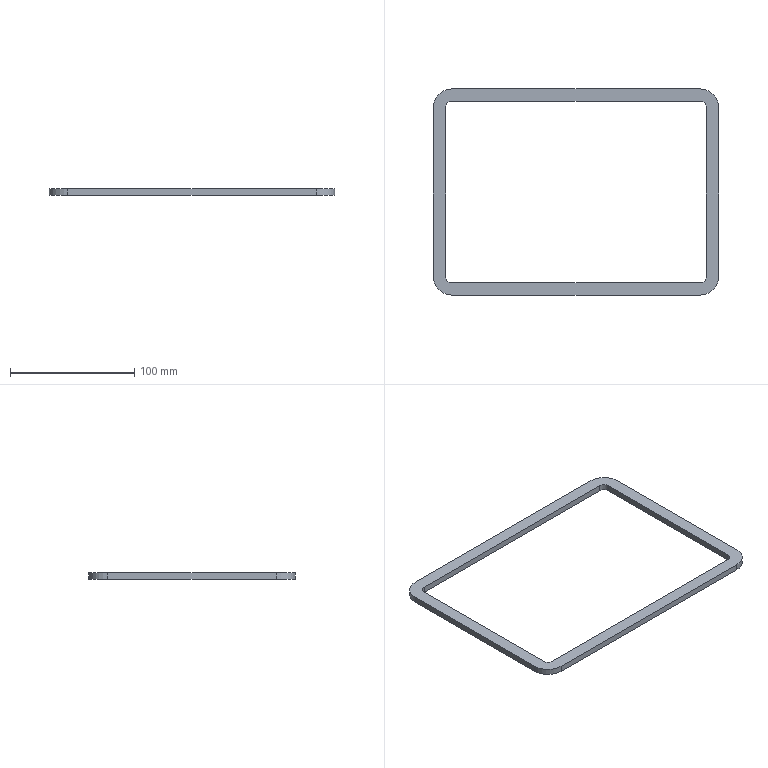Part | SolidWorks | features Fillet 2, Extrusion 1 | 1 solid | 18 faces | box 230 x 166 x 5 mm | volume 36742 mm3 | plane 10 | cylinder 8 | commonest cylinder face diameters 10 x4 30 x4
STEP:
#1=CARTESIAN_POINT('',(-100.,-83.,5.));
#2=VERTEX_POINT('',#1);
#3=CARTESIAN_POINT('',(100.,-83.,5.));
#4=VERTEX_POINT('',#3);
#5=CARTESIAN_POINT('',(-115.,-83.,5.));
#6=DIRECTION('',(1.,0.,0.));
#7=VECTOR('',#6,1000.);
#8=LINE('',#5,#7);
#9=EDGE_CURVE('',#2,#4,#8,.T.);
#10=ORIENTED_EDGE('',*,*,#9,.T.);
#11=CARTESIAN_POINT('',(115.,-68.,5.));
#12=VERTEX_POINT('',#11);
#13=CARTESIAN_POINT('',(100.,-68.,5.));
#14=DIRECTION('',(0.,0.,1.));
#15=DIRECTION('',(1.,0.,0.));
#16=AXIS2_PLACEMENT_3D('',#13,#14,#15);
#17=CIRCLE('',#16,15.);
#18=EDGE_CURVE('',#4,#12,#17,.T.);
#19=ORIENTED_EDGE('',*,*,#18,.T.);
#20=CARTESIAN_POINT('',(115.,68.,5.));
#21=VERTEX_POINT('',#20);
#22=CARTESIAN_POINT('',(115.,83.,5.));
#23=DIRECTION('',(0.,1.,0.));
#24=VECTOR('',#23,1000.);
#25=LINE('',#22,#24);
#26=EDGE_CURVE('',#12,#21,#25,.T.);
#27=ORIENTED_EDGE('',*,*,#26,.T.);
#28=CARTESIAN_POINT('',(100.,83.,5.));
#29=VERTEX_POINT('',#28);
#30=CARTESIAN_POINT('',(100.,68.,5.));
#31=DIRECTION('',(0.,0.,1.));
#32=DIRECTION('',(1.,0.,0.));
#33=AXIS2_PLACEMENT_3D('',#30,#31,#32);
#34=CIRCLE('',#33,15.);
#35=EDGE_CURVE('',#21,#29,#34,.T.);
#36=ORIENTED_EDGE('',*,*,#35,.T.);
#37=CARTESIAN_POINT('',(-100.,83.,5.));
#38=VERTEX_POINT('',#37);
#39=CARTESIAN_POINT('',(-115.,83.,5.));
#40=DIRECTION('',(-1.,0.,0.));
#41=VECTOR('',#40,1000.);
#42=LINE('',#39,#41);
#43=EDGE_CURVE('',#29,#38,#42,.T.);
#44=ORIENTED_EDGE('',*,*,#43,.T.);
#45=CARTESIAN_POINT('',(-115.,68.,5.));
#46=VERTEX_POINT('',#45);
#47=CARTESIAN_POINT('',(-100.,68.,5.));
#48=DIRECTION('',(0.,0.,1.));
#49=DIRECTION('',(1.,0.,0.));
#50=AXIS2_PLACEMENT_3D('',#47,#48,#49);
#51=CIRCLE('',#50,15.);
#52=EDGE_CURVE('',#38,#46,#51,.T.);
#53=ORIENTED_EDGE('',*,*,#52,.T.);
#54=CARTESIAN_POINT('',(-115.,-68.,5.));
#55=VERTEX_POINT('',#54);
#56=CARTESIAN_POINT('',(-115.,83.,5.));
#57=DIRECTION('',(0.,-1.,0.));
#58=VECTOR('',#57,1000.);
#59=LINE('',#56,#58);
#60=EDGE_CURVE('',#46,#55,#59,.T.);
#61=ORIENTED_EDGE('',*,*,#60,.T.);
#62=CARTESIAN_POINT('',(-100.,-68.,5.));
#63=DIRECTION('',(0.,0.,1.));
#64=DIRECTION('',(1.,0.,0.));
#65=AXIS2_PLACEMENT_3D('',#62,#63,#64);
#66=CIRCLE('',#65,15.);
#67=EDGE_CURVE('',#55,#2,#66,.T.);
#68=ORIENTED_EDGE('',*,*,#67,.T.);
#69=EDGE_LOOP('',(#10,#19,#27,#36,#44,#53,#61,#68));
#70=FACE_OUTER_BOUND('',#69,.T.);
#71=CARTESIAN_POINT('',(-100.,-73.,5.));
#72=VERTEX_POINT('',#71);
#73=CARTESIAN_POINT('',(100.,-73.,5.));
#74=VERTEX_POINT('',#73);
#75=CARTESIAN_POINT('',(-105.,-73.,5.));
#76=DIRECTION('',(1.,0.,0.));
#77=VECTOR('',#76,1000.);
#78=LINE('',#75,#77);
#79=EDGE_CURVE('',#72,#74,#78,.T.);
#80=ORIENTED_EDGE('',*,*,#79,.F.);
#81=CARTESIAN_POINT('',(-105.,-68.,5.));
#82=VERTEX_POINT('',#81);
#83=CARTESIAN_POINT('',(-100.,-68.,5.));
#84=DIRECTION('',(0.,0.,-1.));
#85=DIRECTION('',(1.,0.,0.));
#86=AXIS2_PLACEMENT_3D('',#83,#84,#85);
#87=CIRCLE('',#86,5.);
#88=EDGE_CURVE('',#72,#82,#87,.T.);
#89=ORIENTED_EDGE('',*,*,#88,.T.);
#90=CARTESIAN_POINT('',(-105.,68.,5.));
#91=VERTEX_POINT('',#90);
#92=CARTESIAN_POINT('',(-105.,73.,5.));
#93=DIRECTION('',(0.,-1.,0.));
#94=VECTOR('',#93,1000.);
#95=LINE('',#92,#94);
#96=EDGE_CURVE('',#91,#82,#95,.T.);
#97=ORIENTED_EDGE('',*,*,#96,.F.);
#98=CARTESIAN_POINT('',(-100.,73.,5.));
#99=VERTEX_POINT('',#98);
#100=CARTESIAN_POINT('',(-100.,68.,5.));
#101=DIRECTION('',(0.,0.,-1.));
#102=DIRECTION('',(1.,0.,0.));
#103=AXIS2_PLACEMENT_3D('',#100,#101,#102);
#104=CIRCLE('',#103,5.);
#105=EDGE_CURVE('',#91,#99,#104,.T.);
#106=ORIENTED_EDGE('',*,*,#105,.T.);
#107=CARTESIAN_POINT('',(100.,73.,5.));
#108=VERTEX_POINT('',#107);
#109=CARTESIAN_POINT('',(-105.,73.,5.));
#110=DIRECTION('',(-1.,0.,0.));
#111=VECTOR('',#110,1000.);
#112=LINE('',#109,#111);
#113=EDGE_CURVE('',#108,#99,#112,.T.);
#114=ORIENTED_EDGE('',*,*,#113,.F.);
#115=CARTESIAN_POINT('',(105.,68.,5.));
#116=VERTEX_POINT('',#115);
#117=CARTESIAN_POINT('',(100.,68.,5.));
#118=DIRECTION('',(0.,0.,-1.));
#119=DIRECTION('',(1.,0.,0.));
#120=AXIS2_PLACEMENT_3D('',#117,#118,#119);
#121=CIRCLE('',#120,5.);
#122=EDGE_CURVE('',#108,#116,#121,.T.);
#123=ORIENTED_EDGE('',*,*,#122,.T.);
#124=CARTESIAN_POINT('',(105.,-68.,5.));
#125=VERTEX_POINT('',#124);
#126=CARTESIAN_POINT('',(105.,73.,5.));
#127=DIRECTION('',(0.,1.,0.));
#128=VECTOR('',#127,1000.);
#129=LINE('',#126,#128);
#130=EDGE_CURVE('',#125,#116,#129,.T.);
#131=ORIENTED_EDGE('',*,*,#130,.F.);
#132=CARTESIAN_POINT('',(100.,-68.,5.));
#133=DIRECTION('',(0.,0.,-1.));
#134=DIRECTION('',(1.,0.,0.));
#135=AXIS2_PLACEMENT_3D('',#132,#133,#134);
#136=CIRCLE('',#135,5.);
#137=EDGE_CURVE('',#125,#74,#136,.T.);
#138=ORIENTED_EDGE('',*,*,#137,.T.);
#139=EDGE_LOOP('',(#80,#89,#97,#106,#114,#123,#131,#138));
#140=FACE_BOUND('',#139,.T.);
#141=CARTESIAN_POINT('',(0.,0.,5.));
#142=DIRECTION('',(0.,0.,1.));
#143=DIRECTION('',(1.,0.,0.));
#144=AXIS2_PLACEMENT_3D('',#141,#142,#143);
#145=PLANE('',#144);
#146=ADVANCED_FACE('',(#70,#140),#145,.T.);
#147=CARTESIAN_POINT('',(115.,-68.,0.));
#148=VERTEX_POINT('',#147);
#149=CARTESIAN_POINT('',(115.,68.,0.));
#150=VERTEX_POINT('',#149);
#151=CARTESIAN_POINT('',(115.,83.,0.));
#152=DIRECTION('',(0.,1.,0.));
#153=VECTOR('',#152,1000.);
#154=LINE('',#151,#153);
#155=EDGE_CURVE('',#148,#150,#154,.T.);
#156=ORIENTED_EDGE('',*,*,#155,.F.);
#157=CARTESIAN_POINT('',(100.,-83.,0.));
#158=VERTEX_POINT('',#157);
#159=CARTESIAN_POINT('',(100.,-68.,0.));
#160=DIRECTION('',(0.,0.,-1.));
#161=DIRECTION('',(1.,0.,0.));
#162=AXIS2_PLACEMENT_3D('',#159,#160,#161);
#163=CIRCLE('',#162,15.);
#164=EDGE_CURVE('',#148,#158,#163,.T.);
#165=ORIENTED_EDGE('',*,*,#164,.T.);
#166=CARTESIAN_POINT('',(-100.,-83.,0.));
#167=VERTEX_POINT('',#166);
#168=CARTESIAN_POINT('',(-115.,-83.,0.));
#169=DIRECTION('',(1.,0.,0.));
#170=VECTOR('',#169,1000.);
#171=LINE('',#168,#170);
#172=EDGE_CURVE('',#167,#158,#171,.T.);
#173=ORIENTED_EDGE('',*,*,#172,.F.);
#174=CARTESIAN_POINT('',(-115.,-68.,0.));
#175=VERTEX_POINT('',#174);
#176=CARTESIAN_POINT('',(-100.,-68.,0.));
#177=DIRECTION('',(0.,0.,-1.));
#178=DIRECTION('',(1.,0.,0.));
#179=AXIS2_PLACEMENT_3D('',#176,#177,#178);
#180=CIRCLE('',#179,15.);
#181=EDGE_CURVE('',#167,#175,#180,.T.);
#182=ORIENTED_EDGE('',*,*,#181,.T.);
#183=CARTESIAN_POINT('',(-115.,68.,0.));
#184=VERTEX_POINT('',#183);
#185=CARTESIAN_POINT('',(-115.,83.,0.));
#186=DIRECTION('',(0.,-1.,0.));
#187=VECTOR('',#186,1000.);
#188=LINE('',#185,#187);
#189=EDGE_CURVE('',#184,#175,#188,.T.);
#190=ORIENTED_EDGE('',*,*,#189,.F.);
#191=CARTESIAN_POINT('',(-100.,83.,0.));
#192=VERTEX_POINT('',#191);
#193=CARTESIAN_POINT('',(-100.,68.,0.));
#194=DIRECTION('',(0.,0.,-1.));
#195=DIRECTION('',(1.,0.,0.));
#196=AXIS2_PLACEMENT_3D('',#193,#194,#195);
#197=CIRCLE('',#196,15.);
#198=EDGE_CURVE('',#184,#192,#197,.T.);
#199=ORIENTED_EDGE('',*,*,#198,.T.);
#200=CARTESIAN_POINT('',(100.,83.,0.));
#201=VERTEX_POINT('',#200);
#202=CARTESIAN_POINT('',(-115.,83.,0.));
#203=DIRECTION('',(-1.,0.,0.));
#204=VECTOR('',#203,1000.);
#205=LINE('',#202,#204);
#206=EDGE_CURVE('',#201,#192,#205,.T.);
#207=ORIENTED_EDGE('',*,*,#206,.F.);
#208=CARTESIAN_POINT('',(100.,68.,0.));
#209=DIRECTION('',(0.,0.,-1.));
#210=DIRECTION('',(1.,0.,0.));
#211=AXIS2_PLACEMENT_3D('',#208,#209,#210);
#212=CIRCLE('',#211,15.);
#213=EDGE_CURVE('',#201,#150,#212,.T.);
#214=ORIENTED_EDGE('',*,*,#213,.T.);
#215=EDGE_LOOP('',(#156,#165,#173,#182,#190,#199,#207,#214));
#216=FACE_OUTER_BOUND('',#215,.T.);
#217=CARTESIAN_POINT('',(100.,73.,0.));
#218=VERTEX_POINT('',#217);
#219=CARTESIAN_POINT('',(-100.,73.,0.));
#220=VERTEX_POINT('',#219);
#221=CARTESIAN_POINT('',(-105.,73.,0.));
#222=DIRECTION('',(-1.,0.,0.));
#223=VECTOR('',#222,1000.);
#224=LINE('',#221,#223);
#225=EDGE_CURVE('',#218,#220,#224,.T.);
#226=ORIENTED_EDGE('',*,*,#225,.T.);
#227=CARTESIAN_POINT('',(-105.,68.,0.));
#228=VERTEX_POINT('',#227);
#229=CARTESIAN_POINT('',(-100.,68.,0.));
#230=DIRECTION('',(0.,0.,1.));
#231=DIRECTION('',(1.,0.,0.));
#232=AXIS2_PLACEMENT_3D('',#229,#230,#231);
#233=CIRCLE('',#232,5.);
#234=EDGE_CURVE('',#220,#228,#233,.T.);
#235=ORIENTED_EDGE('',*,*,#234,.T.);
#236=CARTESIAN_POINT('',(-105.,-68.,0.));
#237=VERTEX_POINT('',#236);
#238=CARTESIAN_POINT('',(-105.,73.,0.));
#239=DIRECTION('',(0.,-1.,0.));
#240=VECTOR('',#239,1000.);
#241=LINE('',#238,#240);
#242=EDGE_CURVE('',#228,#237,#241,.T.);
#243=ORIENTED_EDGE('',*,*,#242,.T.);
#244=CARTESIAN_POINT('',(-100.,-73.,0.));
#245=VERTEX_POINT('',#244);
#246=CARTESIAN_POINT('',(-100.,-68.,0.));
#247=DIRECTION('',(0.,0.,1.));
#248=DIRECTION('',(1.,0.,0.));
#249=AXIS2_PLACEMENT_3D('',#246,#247,#248);
#250=CIRCLE('',#249,5.);
#251=EDGE_CURVE('',#237,#245,#250,.T.);
#252=ORIENTED_EDGE('',*,*,#251,.T.);
#253=CARTESIAN_POINT('',(100.,-73.,0.));
#254=VERTEX_POINT('',#253);
#255=CARTESIAN_POINT('',(-105.,-73.,0.));
#256=DIRECTION('',(1.,0.,0.));
#257=VECTOR('',#256,1000.);
#258=LINE('',#255,#257);
#259=EDGE_CURVE('',#245,#254,#258,.T.);
#260=ORIENTED_EDGE('',*,*,#259,.T.);
#261=CARTESIAN_POINT('',(105.,-68.,0.));
#262=VERTEX_POINT('',#261);
#263=CARTESIAN_POINT('',(100.,-68.,0.));
#264=DIRECTION('',(0.,0.,1.));
#265=DIRECTION('',(1.,0.,0.));
#266=AXIS2_PLACEMENT_3D('',#263,#264,#265);
#267=CIRCLE('',#266,5.);
#268=EDGE_CURVE('',#254,#262,#267,.T.);
#269=ORIENTED_EDGE('',*,*,#268,.T.);
#270=CARTESIAN_POINT('',(105.,68.,0.));
#271=VERTEX_POINT('',#270);
#272=CARTESIAN_POINT('',(105.,73.,0.));
#273=DIRECTION('',(0.,1.,0.));
#274=VECTOR('',#273,1000.);
#275=LINE('',#272,#274);
#276=EDGE_CURVE('',#262,#271,#275,.T.);
#277=ORIENTED_EDGE('',*,*,#276,.T.);
#278=CARTESIAN_POINT('',(100.,68.,0.));
#279=DIRECTION('',(0.,0.,1.));
#280=DIRECTION('',(1.,0.,0.));
#281=AXIS2_PLACEMENT_3D('',#278,#279,#280);
#282=CIRCLE('',#281,5.);
#283=EDGE_CURVE('',#271,#218,#282,.T.);
#284=ORIENTED_EDGE('',*,*,#283,.T.);
#285=EDGE_LOOP('',(#226,#235,#243,#252,#260,#269,#277,#284));
#286=FACE_BOUND('',#285,.T.);
#287=CARTESIAN_POINT('',(0.,0.,0.));
#288=DIRECTION('',(0.,0.,1.));
#289=DIRECTION('',(1.,0.,0.));
#290=AXIS2_PLACEMENT_3D('',#287,#288,#289);
#291=PLANE('',#290);
#292=ADVANCED_FACE('',(#216,#286),#291,.F.);
#293=ORIENTED_EDGE('',*,*,#60,.F.);
#294=CARTESIAN_POINT('',(-115.,68.,5.));
#295=DIRECTION('',(0.,0.,-1.));
#296=VECTOR('',#295,1000.);
#297=LINE('',#294,#296);
#298=EDGE_CURVE('',#46,#184,#297,.T.);
#299=ORIENTED_EDGE('',*,*,#298,.T.);
#300=ORIENTED_EDGE('',*,*,#189,.T.);
#301=CARTESIAN_POINT('',(-115.,-68.,5.));
#302=DIRECTION('',(0.,0.,1.));
#303=VECTOR('',#302,1000.);
#304=LINE('',#301,#303);
#305=EDGE_CURVE('',#175,#55,#304,.T.);
#306=ORIENTED_EDGE('',*,*,#305,.T.);
#307=EDGE_LOOP('',(#293,#299,#300,#306));
#308=FACE_OUTER_BOUND('',#307,.T.);
#309=CARTESIAN_POINT('',(-115.,83.,5.));
#310=DIRECTION('',(1.,0.,0.));
#311=DIRECTION('',(0.,1.,0.));
#312=AXIS2_PLACEMENT_3D('',#309,#310,#311);
#313=PLANE('',#312);
#314=ADVANCED_FACE('',(#308),#313,.F.);
#315=ORIENTED_EDGE('',*,*,#172,.T.);
#316=CARTESIAN_POINT('',(100.,-83.,5.));
#317=DIRECTION('',(0.,0.,1.));
#318=VECTOR('',#317,1000.);
#319=LINE('',#316,#318);
#320=EDGE_CURVE('',#158,#4,#319,.T.);
#321=ORIENTED_EDGE('',*,*,#320,.T.);
#322=ORIENTED_EDGE('',*,*,#9,.F.);
#323=CARTESIAN_POINT('',(-100.,-83.,5.));
#324=DIRECTION('',(0.,0.,-1.));
#325=VECTOR('',#324,1000.);
#326=LINE('',#323,#325);
#327=EDGE_CURVE('',#2,#167,#326,.T.);
#328=ORIENTED_EDGE('',*,*,#327,.T.);
#329=EDGE_LOOP('',(#315,#321,#322,#328));
#330=FACE_OUTER_BOUND('',#329,.T.);
#331=CARTESIAN_POINT('',(-115.,-83.,5.));
#332=DIRECTION('',(0.,1.,0.));
#333=DIRECTION('',(0.,0.,1.));
#334=AXIS2_PLACEMENT_3D('',#331,#332,#333);
#335=PLANE('',#334);
#336=ADVANCED_FACE('',(#330),#335,.F.);
#337=ORIENTED_EDGE('',*,*,#26,.F.);
#338=CARTESIAN_POINT('',(115.,-68.,5.));
#339=DIRECTION('',(0.,0.,-1.));
#340=VECTOR('',#339,1000.);
#341=LINE('',#338,#340);
#342=EDGE_CURVE('',#12,#148,#341,.T.);
#343=ORIENTED_EDGE('',*,*,#342,.T.);
#344=ORIENTED_EDGE('',*,*,#155,.T.);
#345=CARTESIAN_POINT('',(115.,68.,5.));
#346=DIRECTION('',(0.,0.,1.));
#347=VECTOR('',#346,1000.);
#348=LINE('',#345,#347);
#349=EDGE_CURVE('',#150,#21,#348,.T.);
#350=ORIENTED_EDGE('',*,*,#349,.T.);
#351=EDGE_LOOP('',(#337,#343,#344,#350));
#352=FACE_OUTER_BOUND('',#351,.T.);
#353=CARTESIAN_POINT('',(115.,83.,5.));
#354=DIRECTION('',(-1.,0.,0.));
#355=DIRECTION('',(0.,-1.,0.));
#356=AXIS2_PLACEMENT_3D('',#353,#354,#355);
#357=PLANE('',#356);
#358=ADVANCED_FACE('',(#352),#357,.F.);
#359=ORIENTED_EDGE('',*,*,#43,.F.);
#360=CARTESIAN_POINT('',(100.,83.,5.));
#361=DIRECTION('',(0.,0.,-1.));
#362=VECTOR('',#361,1000.);
#363=LINE('',#360,#362);
#364=EDGE_CURVE('',#29,#201,#363,.T.);
#365=ORIENTED_EDGE('',*,*,#364,.T.);
#366=ORIENTED_EDGE('',*,*,#206,.T.);
#367=CARTESIAN_POINT('',(-100.,83.,5.));
#368=DIRECTION('',(0.,0.,1.));
#369=VECTOR('',#368,1000.);
#370=LINE('',#367,#369);
#371=EDGE_CURVE('',#192,#38,#370,.T.);
#372=ORIENTED_EDGE('',*,*,#371,.T.);
#373=EDGE_LOOP('',(#359,#365,#366,#372));
#374=FACE_OUTER_BOUND('',#373,.T.);
#375=CARTESIAN_POINT('',(-115.,83.,5.));
#376=DIRECTION('',(0.,-1.,0.));
#377=DIRECTION('',(0.,0.,-1.));
#378=AXIS2_PLACEMENT_3D('',#375,#376,#377);
#379=PLANE('',#378);
#380=ADVANCED_FACE('',(#374),#379,.F.);
#381=ORIENTED_EDGE('',*,*,#242,.F.);
#382=CARTESIAN_POINT('',(-105.,68.,5.));
#383=DIRECTION('',(0.,0.,1.));
#384=VECTOR('',#383,1000.);
#385=LINE('',#382,#384);
#386=EDGE_CURVE('',#228,#91,#385,.T.);
#387=ORIENTED_EDGE('',*,*,#386,.T.);
#388=ORIENTED_EDGE('',*,*,#96,.T.);
#389=CARTESIAN_POINT('',(-105.,-68.,0.));
#390=DIRECTION('',(0.,0.,-1.));
#391=VECTOR('',#390,1000.);
#392=LINE('',#389,#391);
#393=EDGE_CURVE('',#82,#237,#392,.T.);
#394=ORIENTED_EDGE('',*,*,#393,.T.);
#395=EDGE_LOOP('',(#381,#387,#388,#394));
#396=FACE_OUTER_BOUND('',#395,.T.);
#397=CARTESIAN_POINT('',(-105.,73.,5.));
#398=DIRECTION('',(1.,0.,0.));
#399=DIRECTION('',(0.,1.,0.));
#400=AXIS2_PLACEMENT_3D('',#397,#398,#399);
#401=PLANE('',#400);
#402=ADVANCED_FACE('',(#396),#401,.T.);
#403=ORIENTED_EDGE('',*,*,#79,.T.);
#404=CARTESIAN_POINT('',(100.,-73.,0.));
#405=DIRECTION('',(0.,0.,-1.));
#406=VECTOR('',#405,1000.);
#407=LINE('',#404,#406);
#408=EDGE_CURVE('',#74,#254,#407,.T.);
#409=ORIENTED_EDGE('',*,*,#408,.T.);
#410=ORIENTED_EDGE('',*,*,#259,.F.);
#411=CARTESIAN_POINT('',(-100.,-73.,5.));
#412=DIRECTION('',(0.,0.,1.));
#413=VECTOR('',#412,1000.);
#414=LINE('',#411,#413);
#415=EDGE_CURVE('',#245,#72,#414,.T.);
#416=ORIENTED_EDGE('',*,*,#415,.T.);
#417=EDGE_LOOP('',(#403,#409,#410,#416));
#418=FACE_OUTER_BOUND('',#417,.T.);
#419=CARTESIAN_POINT('',(-105.,-73.,5.));
#420=DIRECTION('',(0.,1.,0.));
#421=DIRECTION('',(-1.,0.,0.));
#422=AXIS2_PLACEMENT_3D('',#419,#420,#421);
#423=PLANE('',#422);
#424=ADVANCED_FACE('',(#418),#423,.T.);
#425=ORIENTED_EDGE('',*,*,#130,.T.);
#426=CARTESIAN_POINT('',(105.,68.,0.));
#427=DIRECTION('',(0.,0.,-1.));
#428=VECTOR('',#427,1000.);
#429=LINE('',#426,#428);
#430=EDGE_CURVE('',#116,#271,#429,.T.);
#431=ORIENTED_EDGE('',*,*,#430,.T.);
#432=ORIENTED_EDGE('',*,*,#276,.F.);
#433=CARTESIAN_POINT('',(105.,-68.,5.));
#434=DIRECTION('',(0.,0.,1.));
#435=VECTOR('',#434,1000.);
#436=LINE('',#433,#435);
#437=EDGE_CURVE('',#262,#125,#436,.T.);
#438=ORIENTED_EDGE('',*,*,#437,.T.);
#439=EDGE_LOOP('',(#425,#431,#432,#438));
#440=FACE_OUTER_BOUND('',#439,.T.);
#441=CARTESIAN_POINT('',(105.,73.,5.));
#442=DIRECTION('',(-1.,0.,0.));
#443=DIRECTION('',(0.,-1.,0.));
#444=AXIS2_PLACEMENT_3D('',#441,#442,#443);
#445=PLANE('',#444);
#446=ADVANCED_FACE('',(#440),#445,.T.);
#447=ORIENTED_EDGE('',*,*,#113,.T.);
#448=CARTESIAN_POINT('',(-100.,73.,0.));
#449=DIRECTION('',(0.,0.,-1.));
#450=VECTOR('',#449,1000.);
#451=LINE('',#448,#450);
#452=EDGE_CURVE('',#99,#220,#451,.T.);
#453=ORIENTED_EDGE('',*,*,#452,.T.);
#454=ORIENTED_EDGE('',*,*,#225,.F.);
#455=CARTESIAN_POINT('',(100.,73.,5.));
#456=DIRECTION('',(0.,0.,1.));
#457=VECTOR('',#456,1000.);
#458=LINE('',#455,#457);
#459=EDGE_CURVE('',#218,#108,#458,.T.);
#460=ORIENTED_EDGE('',*,*,#459,.T.);
#461=EDGE_LOOP('',(#447,#453,#454,#460));
#462=FACE_OUTER_BOUND('',#461,.T.);
#463=CARTESIAN_POINT('',(-105.,73.,5.));
#464=DIRECTION('',(0.,-1.,0.));
#465=DIRECTION('',(0.,0.,-1.));
#466=AXIS2_PLACEMENT_3D('',#463,#464,#465);
#467=PLANE('',#466);
#468=ADVANCED_FACE('',(#462),#467,.T.);
#469=ORIENTED_EDGE('',*,*,#105,.F.);
#470=ORIENTED_EDGE('',*,*,#386,.F.);
#471=ORIENTED_EDGE('',*,*,#234,.F.);
#472=ORIENTED_EDGE('',*,*,#452,.F.);
#473=EDGE_LOOP('',(#469,#470,#471,#472));
#474=FACE_OUTER_BOUND('',#473,.T.);
#475=CARTESIAN_POINT('',(-100.,68.,5.));
#476=DIRECTION('',(0.,0.,1.));
#477=DIRECTION('',(1.,0.,0.));
#478=AXIS2_PLACEMENT_3D('',#475,#476,#477);
#479=CYLINDRICAL_SURFACE('',#478,5.);
#480=ADVANCED_FACE('',(#474),#479,.F.);
#481=ORIENTED_EDGE('',*,*,#122,.F.);
#482=ORIENTED_EDGE('',*,*,#459,.F.);
#483=ORIENTED_EDGE('',*,*,#283,.F.);
#484=ORIENTED_EDGE('',*,*,#430,.F.);
#485=EDGE_LOOP('',(#481,#482,#483,#484));
#486=FACE_OUTER_BOUND('',#485,.T.);
#487=CARTESIAN_POINT('',(100.,68.,5.));
#488=DIRECTION('',(0.,0.,1.));
#489=DIRECTION('',(1.,0.,0.));
#490=AXIS2_PLACEMENT_3D('',#487,#488,#489);
#491=CYLINDRICAL_SURFACE('',#490,5.);
#492=ADVANCED_FACE('',(#486),#491,.F.);
#493=ORIENTED_EDGE('',*,*,#137,.F.);
#494=ORIENTED_EDGE('',*,*,#437,.F.);
#495=ORIENTED_EDGE('',*,*,#268,.F.);
#496=ORIENTED_EDGE('',*,*,#408,.F.);
#497=EDGE_LOOP('',(#493,#494,#495,#496));
#498=FACE_OUTER_BOUND('',#497,.T.);
#499=CARTESIAN_POINT('',(100.,-68.,5.));
#500=DIRECTION('',(0.,0.,1.));
#501=DIRECTION('',(1.,0.,0.));
#502=AXIS2_PLACEMENT_3D('',#499,#500,#501);
#503=CYLINDRICAL_SURFACE('',#502,5.);
#504=ADVANCED_FACE('',(#498),#503,.F.);
#505=ORIENTED_EDGE('',*,*,#88,.F.);
#506=ORIENTED_EDGE('',*,*,#415,.F.);
#507=ORIENTED_EDGE('',*,*,#251,.F.);
#508=ORIENTED_EDGE('',*,*,#393,.F.);
#509=EDGE_LOOP('',(#505,#506,#507,#508));
#510=FACE_OUTER_BOUND('',#509,.T.);
#511=CARTESIAN_POINT('',(-100.,-68.,5.));
#512=DIRECTION('',(0.,0.,1.));
#513=DIRECTION('',(1.,0.,0.));
#514=AXIS2_PLACEMENT_3D('',#511,#512,#513);
#515=CYLINDRICAL_SURFACE('',#514,5.);
#516=ADVANCED_FACE('',(#510),#515,.F.);
#517=ORIENTED_EDGE('',*,*,#18,.F.);
#518=ORIENTED_EDGE('',*,*,#320,.F.);
#519=ORIENTED_EDGE('',*,*,#164,.F.);
#520=ORIENTED_EDGE('',*,*,#342,.F.);
#521=EDGE_LOOP('',(#517,#518,#519,#520));
#522=FACE_OUTER_BOUND('',#521,.T.);
#523=CARTESIAN_POINT('',(100.,-68.,5.));
#524=DIRECTION('',(0.,0.,-1.));
#525=DIRECTION('',(-1.,0.,0.));
#526=AXIS2_PLACEMENT_3D('',#523,#524,#525);
#527=CYLINDRICAL_SURFACE('',#526,15.);
#528=ADVANCED_FACE('',(#522),#527,.T.);
#529=ORIENTED_EDGE('',*,*,#35,.F.);
#530=ORIENTED_EDGE('',*,*,#349,.F.);
#531=ORIENTED_EDGE('',*,*,#213,.F.);
#532=ORIENTED_EDGE('',*,*,#364,.F.);
#533=EDGE_LOOP('',(#529,#530,#531,#532));
#534=FACE_OUTER_BOUND('',#533,.T.);
#535=CARTESIAN_POINT('',(100.,68.,5.));
#536=DIRECTION('',(0.,0.,-1.));
#537=DIRECTION('',(-1.,0.,0.));
#538=AXIS2_PLACEMENT_3D('',#535,#536,#537);
#539=CYLINDRICAL_SURFACE('',#538,15.);
#540=ADVANCED_FACE('',(#534),#539,.T.);
#541=ORIENTED_EDGE('',*,*,#52,.F.);
#542=ORIENTED_EDGE('',*,*,#371,.F.);
#543=ORIENTED_EDGE('',*,*,#198,.F.);
#544=ORIENTED_EDGE('',*,*,#298,.F.);
#545=EDGE_LOOP('',(#541,#542,#543,#544));
#546=FACE_OUTER_BOUND('',#545,.T.);
#547=CARTESIAN_POINT('',(-100.,68.,5.));
#548=DIRECTION('',(0.,0.,-1.));
#549=DIRECTION('',(-1.,0.,0.));
#550=AXIS2_PLACEMENT_3D('',#547,#548,#549);
#551=CYLINDRICAL_SURFACE('',#550,15.);
#552=ADVANCED_FACE('',(#546),#551,.T.);
#553=ORIENTED_EDGE('',*,*,#67,.F.);
#554=ORIENTED_EDGE('',*,*,#305,.F.);
#555=ORIENTED_EDGE('',*,*,#181,.F.);
#556=ORIENTED_EDGE('',*,*,#327,.F.);
#557=EDGE_LOOP('',(#553,#554,#555,#556));
#558=FACE_OUTER_BOUND('',#557,.T.);
#559=CARTESIAN_POINT('',(-100.,-68.,5.));
#560=DIRECTION('',(0.,0.,-1.));
#561=DIRECTION('',(-1.,0.,0.));
#562=AXIS2_PLACEMENT_3D('',#559,#560,#561);
#563=CYLINDRICAL_SURFACE('',#562,15.);
#564=ADVANCED_FACE('',(#558),#563,.T.);
#565=CLOSED_SHELL('',(#146,#292,#314,#336,#358,#380,#402,#424,#446,#468,#480,#492,#504,#516,#528,#540,#552,#564));
#566=MANIFOLD_SOLID_BREP('',#565);
#567=CARTESIAN_POINT('',(0.,0.,0.));
#568=DIRECTION('',(0.,0.,1.));
#569=DIRECTION('',(1.,0.,0.));
#570=AXIS2_PLACEMENT_3D('',#567,#568,#569);
#571=(LENGTH_UNIT()NAMED_UNIT(*)SI_UNIT(.MILLI.,.METRE.));
#572=UNCERTAINTY_MEASURE_WITH_UNIT(LENGTH_MEASURE(0.00001),#571,'','');
#573=(NAMED_UNIT(*)PLANE_ANGLE_UNIT()SI_UNIT($,.RADIAN.));
#574=(NAMED_UNIT(*)SI_UNIT($,.STERADIAN.)SOLID_ANGLE_UNIT());
#575=(GEOMETRIC_REPRESENTATION_CONTEXT(3)GLOBAL_UNCERTAINTY_ASSIGNED_CONTEXT((#572))GLOBAL_UNIT_ASSIGNED_CONTEXT((#571,#573,#574))REPRESENTATION_CONTEXT('',''));
#576=ADVANCED_BREP_SHAPE_REPRESENTATION('',(#566,#570),#575);